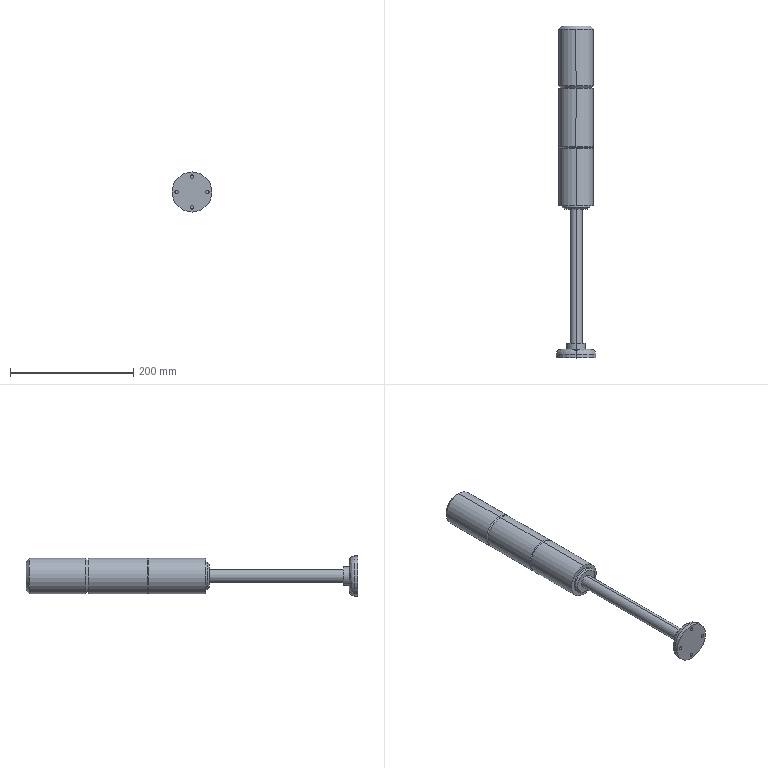Part | STEP file | Alarm light | 1 solid | 52 faces | box 65 x 539.374 x 65 mm | volume 871558 mm3 | cylinder 30 | plane 12 | cone 8 | spline 2 | commonest cylinder face diameters 5.5 x8 9.9 x8 57 x6 20.81 x2 30 x2 44.44 x2